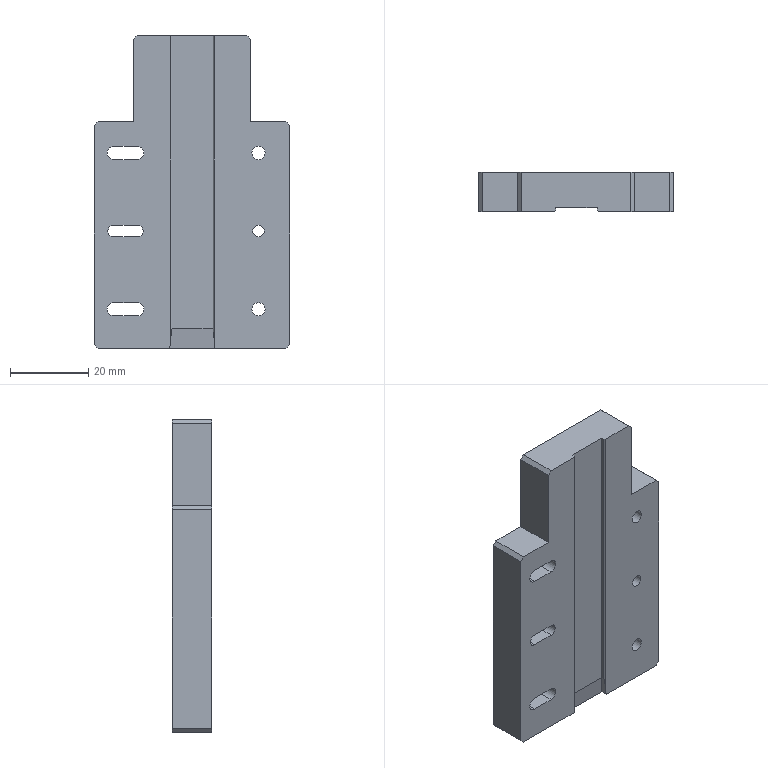CAM job | NX | 3+2 milling, drilling | part box 50 x 10 x 80 mm | stock box 55 x 12 x 85 mm
Tools:
number,name,description,diameter,corner_radius,flute_length,length,flutes
4,D4,平底铣刀-粗,4.0,0.0,25.0,75.0,2
9,D10,平底铣刀-粗,10.0,0.0,35.0,75.0,2
18,D2-J,平底铣刀-精,2.0,0.0,50.0,75.0,2
11,D4-J,平底铣刀-精,4.0,0.0,50.0,75.0,2
7,D6-J,平底铣刀-精,6.0,0.0,25.0,75.0,2
10,D10-J,平底铣刀-精,10.0,0.0,35.0,75.0,2
2,D6倒角刀,倒角刀,6.0,0.0,3.0,25.0,2
19,D3铰刀,Drilling Tool,3.0,0.0,75.0,100.0,6
13,ZT3.4,钻头,3.4,0.0,35.0,50.0,2
17,ZT2.9,Drilling Tool,2.9,0.0,35.0,50.0,2
Operations:
program,operation,operation_type,tool,method,geometry_group,spindle_rpm,surface_speed,feed_per_tooth,feed_cut,feed_plunge,cut_length_mm,path_length_mm,cut_time_min,machine_time_min
B,AUTOFACEFINISH_COPY,FaceMilling,D10-J,SIDEFINISH-DEPTHK-STEPG,W-B,8000.0,251.327,0.0625,1000.0,100.0,3922.385,4372.928,3.922,3.967
B,AUTOFACEFINISH_COPY_COPY,FaceMilling,D10-J,SIDEFINISH-DEPTHK-STEPG,W-B,8000.0,251.327,0.0625,1000.0,100.0,980.596,1076.596,0.9806,0.9902
B,CAVITYROUGH-MID_COPY,CavityMilling,D4,LAYERROUGH-DEPTHK-STEPG,W-B,8000.0,150.792,0.1875,3000.0,100.0,1526.918,1610.38,0.509,0.5197
B,DRILLCHAMFER_2,Operation,D6倒角刀,METHOD,W-B,8000.0,150.796,0.0625,1000.0,0.0,4.8,109.6,0.0048,0.0153
B,DRILLCHAMFER_3,Operation,D6倒角刀,METHOD,W-B,8000.0,150.796,0.0625,1000.0,0.0,10.0,163.112,0.01,0.0253
B,PLANEDEBURR6X45L_COPY,SurfaceContour,D6倒角刀,CLIMB_CHAMFER-DEPTH0-STEPG,W-B,6500.0,122.519,0.1154,1500.0,100.0,358.331,847.661,0.2389,0.2878
B,FLOORWALLCHAMFER_COPY,VolumeBased25DMillingOperation,D6倒角刀,CLIMB_CHAMFER-DEPTH0-STEPG,W-B,6500.0,122.519,0.1154,1500.0,100.0,179.539,286.525,0.1197,0.1304
B,FLOORWALLFINISHFLOOR-MID_COPY,VolumeBased25DMillingOperation,D4-J,FINISHSTEPDEPTHOFF,W-B,8000.0,100.528,0.05,800.0,100.0,321.839,344.439,0.4023,0.4046
B,FLOORWALLFINISHWALL-MID-SELFLOOR_COPY,VolumeBased25DMillingOperation,D4-J,SIDEFINISH-DEPTHK-STEPG,W-B,8000.0,100.528,0.05,800.0,100.0,167.845,196.594,0.2098,0.2127
B,CURVEPOINTDRIVE_COPY,SurfaceContour,D4-J,CLIMB_CHAMFER-DEPTH0-STEPG,B,5000.0,94.245,0.25,2500.0,100.0,33.692,235.704,0.0135,0.0337
B,ZLEVELFINISHZIGZAG_COPY,ZLevelMilling,D4-J,ZLEVELCLIMB-DEPTHK-STEPG,W-B,7000.0,131.943,0.1786,2500.0,100.0,961.17,990.229,0.3845,0.3874
A,DYNAMICROUGHD10_COPY,CavityMilling,D10,DYNAMICROUGH-DEPTHK-STEPK,W-A,8000.0,251.32,0.25,4000.0,100.0,3915.311,4031.311,0.9788,0.9904
A,TOPFACE_1,FaceMilling,D10-J,SIDEFINISH-DEPTHK-STEPG,W-A,4500.0,1385.0,0.1667,1500.0,100.0,960.797,1056.797,0.6405,0.6501
A,SPOTDRILL-DEPTH0.8,Operation,D6倒角刀,NONE,W-A,8000.0,150.796,0.0312,500.0,90.0,5.4,152.85,0.0108,0.0255
A,THRUHOLE-PILOT3.0,Operation,ZT2.9,NONE,W-A,3200.0,29.154,0.0312,200.0,90.0,14.837,129.674,0.0742,0.0857
A,CSINKDRILL_SEG0,Operation,ZT3.4,NONE,W-A,2800.0,29.908,0.0179,100.0,90.0,28.043,197.098,0.2804,0.2973
A,BLINDSLOTROUGH,VolumeBased25DMillingOperation,D4,METHOD,W-A,9000.0,113.097,0.0667,1200.0,100.0,887.452,1134.455,0.7395,0.7642
A,THRUSLOTROUGH_1,VolumeBased25DMillingOperation,D2-J,METHOD,W-A,12000.0,75.398,0.025,600.0,100.0,1588.071,1696.571,2.647,2.658
A,SLOTROUGH_1,VolumeBased25DMillingOperation,D2-J,METHOD,W-A,12000.0,75.398,0.025,600.0,100.0,2210.815,2477.818,3.685,3.711
A,HOLEROUGHD4_1,CylinderMilling,D4,NONE,W-A,8000.0,100.531,0.075,1200.0,100.0,286.846,535.846,0.239,0.2639
A,HOLEFINISHD4_1,CylinderMilling,D4-J,FINISHSTEPDEPTHOFF,W-A,8000.0,100.531,0.0312,500.0,100.0,43.871,292.871,0.0877,0.1126
A,SLOTFINISH,VolumeBased25DMillingOperation,D4-J,METHOD,W-A,8000.0,100.531,0.0312,500.0,100.0,44.165,302.175,0.0883,0.1141
A,ZLEVELSMOOTHCORNERD2REF6_COPY,ZLevelMilling,D2-J,LAYERFINISH-DEPTHK-STEPG,W-A,8000.0,50.264,0.05,800.0,100.0,2703.595,2955.395,3.38,3.405
A,SLOTFINISH_4,VolumeBased25DMillingOperation,D2-J,METHOD,W-A,6000.0,113.0,0.0167,200.0,100.0,149.012,452.516,0.7451,0.7754
A,SELBODYONLY,SurfaceContour,D6倒角刀,METHOD,W-A,8000.0,150.796,0.1875,3000.0,100.0,362.56,829.909,0.1209,0.1676
A,DRILLCHAMFER_1,Operation,D6倒角刀,METHOD,W-A,8000.0,150.796,0.0312,500.0,0.0,4.8,109.6,0.0096,0.0201
A,MILLCHAMFER_1,PlanarMilling,D6倒角刀,NONE,W-A,8000.0,150.796,0.0312,500.0,100.0,58.511,295.087,0.117,0.1407
A,REAM,Operation,D3铰刀,METHOD,W-A,500.0,4.712,0.0167,50.0,0.0,12.0,124.0,0.24,0.2512
A,SLOTFINISH_3,VolumeBased25DMillingOperation,D2-J,METHOD,W-A,8000.0,50.266,0.0125,200.0,100.0,87.164,225.764,0.4358,0.4497
A,PROFILESEMI_2,VolumeBased25DMillingOperation,D6-J,METHOD,W-A,9000.0,169.646,0.0667,1200.0,100.0,277.676,396.676,0.2314,0.2433